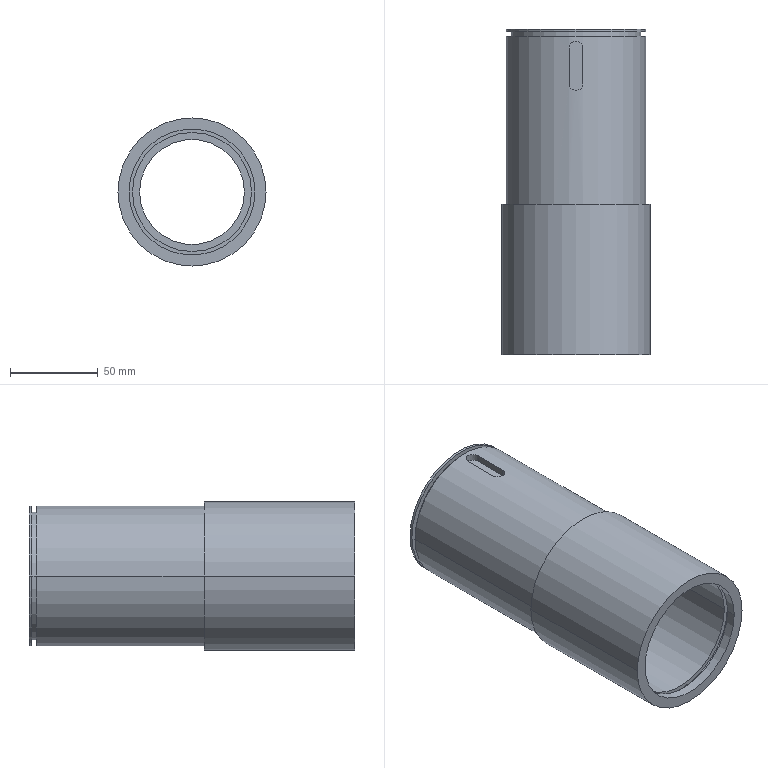Part | SolidWorks | features BaseBody 1 | 1 solid | 32 faces | box 84.6 x 186 x 84.6 mm | volume 291294 mm3 | cylinder 20 | plane 12 | commonest cylinder face diameters 72 x4 80 x4 8 x2 60 x2 68 x2 74 x2
STEP:
#1=CARTESIAN_POINT('',(34.,60.,0.));
#2=VERTEX_POINT('',#1);
#3=CARTESIAN_POINT('',(-34.,60.,0.));
#4=VERTEX_POINT('',#3);
#5=CARTESIAN_POINT('',(0.,60.,0.));
#6=DIRECTION('',(0.,1.,0.));
#7=DIRECTION('',(-1.,0.,0.));
#8=AXIS2_PLACEMENT_3D('',#5,#6,#7);
#9=CIRCLE('',#8,34.);
#10=EDGE_CURVE('',#2,#4,#9,.T.);
#11=ORIENTED_EDGE('',*,*,#10,.F.);
#12=CARTESIAN_POINT('',(34.,172.,0.));
#13=VERTEX_POINT('',#12);
#14=CARTESIAN_POINT('',(34.,0.,0.));
#15=DIRECTION('',(0.,1.,0.));
#16=VECTOR('',#15,1000.);
#17=LINE('',#14,#16);
#18=EDGE_CURVE('',#2,#13,#17,.T.);
#19=ORIENTED_EDGE('',*,*,#18,.T.);
#20=CARTESIAN_POINT('',(-34.,172.,0.));
#21=VERTEX_POINT('',#20);
#22=CARTESIAN_POINT('',(0.,172.,0.));
#23=DIRECTION('',(0.,-1.,0.));
#24=DIRECTION('',(-1.,0.,0.));
#25=AXIS2_PLACEMENT_3D('',#22,#23,#24);
#26=CIRCLE('',#25,34.);
#27=EDGE_CURVE('',#21,#13,#26,.T.);
#28=ORIENTED_EDGE('',*,*,#27,.F.);
#29=CARTESIAN_POINT('',(-34.,0.,0.));
#30=DIRECTION('',(0.,1.,0.));
#31=VECTOR('',#30,1000.);
#32=LINE('',#29,#31);
#33=EDGE_CURVE('',#4,#21,#32,.T.);
#34=ORIENTED_EDGE('',*,*,#33,.F.);
#35=EDGE_LOOP('',(#11,#19,#28,#34));
#36=FACE_OUTER_BOUND('',#35,.T.);
#37=CARTESIAN_POINT('',(0.,0.,0.));
#38=DIRECTION('',(0.,1.,0.));
#39=DIRECTION('',(-1.,0.,0.));
#40=AXIS2_PLACEMENT_3D('',#37,#38,#39);
#41=CYLINDRICAL_SURFACE('',#40,34.);
#42=ADVANCED_FACE('',(#36),#41,.F.);
#43=CARTESIAN_POINT('',(-36.,60.,0.));
#44=VERTEX_POINT('',#43);
#45=CARTESIAN_POINT('',(36.,60.,0.));
#46=VERTEX_POINT('',#45);
#47=CARTESIAN_POINT('',(0.,60.,0.));
#48=DIRECTION('',(0.,-1.,0.));
#49=DIRECTION('',(1.,0.,0.));
#50=AXIS2_PLACEMENT_3D('',#47,#48,#49);
#51=CIRCLE('',#50,36.);
#52=EDGE_CURVE('',#44,#46,#51,.T.);
#53=ORIENTED_EDGE('',*,*,#52,.F.);
#54=CARTESIAN_POINT('',(-36.,8.,0.));
#55=VERTEX_POINT('',#54);
#56=CARTESIAN_POINT('',(-36.,60.,0.));
#57=DIRECTION('',(0.,-1.,0.));
#58=VECTOR('',#57,1000.);
#59=LINE('',#56,#58);
#60=EDGE_CURVE('',#44,#55,#59,.T.);
#61=ORIENTED_EDGE('',*,*,#60,.T.);
#62=CARTESIAN_POINT('',(36.,8.,0.));
#63=VERTEX_POINT('',#62);
#64=CARTESIAN_POINT('',(0.,8.,0.));
#65=DIRECTION('',(0.,1.,0.));
#66=DIRECTION('',(1.,0.,0.));
#67=AXIS2_PLACEMENT_3D('',#64,#65,#66);
#68=CIRCLE('',#67,36.);
#69=EDGE_CURVE('',#63,#55,#68,.T.);
#70=ORIENTED_EDGE('',*,*,#69,.F.);
#71=CARTESIAN_POINT('',(36.,60.,0.));
#72=DIRECTION('',(0.,-1.,0.));
#73=VECTOR('',#72,1000.);
#74=LINE('',#71,#73);
#75=EDGE_CURVE('',#46,#63,#74,.T.);
#76=ORIENTED_EDGE('',*,*,#75,.F.);
#77=EDGE_LOOP('',(#53,#61,#70,#76));
#78=FACE_OUTER_BOUND('',#77,.T.);
#79=CARTESIAN_POINT('',(0.,60.,0.));
#80=DIRECTION('',(0.,-1.,0.));
#81=DIRECTION('',(1.,0.,0.));
#82=AXIS2_PLACEMENT_3D('',#79,#80,#81);
#83=CYLINDRICAL_SURFACE('',#82,36.);
#84=ADVANCED_FACE('',(#78),#83,.F.);
#85=CARTESIAN_POINT('',(-30.,172.,0.));
#86=VERTEX_POINT('',#85);
#87=CARTESIAN_POINT('',(30.,172.,0.));
#88=VERTEX_POINT('',#87);
#89=CARTESIAN_POINT('',(0.,172.,0.));
#90=DIRECTION('',(0.,-1.,0.));
#91=DIRECTION('',(-1.,0.,0.));
#92=AXIS2_PLACEMENT_3D('',#89,#90,#91);
#93=CIRCLE('',#92,30.);
#94=EDGE_CURVE('',#86,#88,#93,.T.);
#95=ORIENTED_EDGE('',*,*,#94,.T.);
#96=CARTESIAN_POINT('',(30.,186.,0.));
#97=VERTEX_POINT('',#96);
#98=CARTESIAN_POINT('',(30.,87.,0.));
#99=DIRECTION('',(0.,1.,0.));
#100=VECTOR('',#99,1000.);
#101=LINE('',#98,#100);
#102=EDGE_CURVE('',#88,#97,#101,.T.);
#103=ORIENTED_EDGE('',*,*,#102,.T.);
#104=CARTESIAN_POINT('',(-30.,186.,0.));
#105=VERTEX_POINT('',#104);
#106=CARTESIAN_POINT('',(0.,186.,0.));
#107=DIRECTION('',(0.,-1.,0.));
#108=DIRECTION('',(-1.,0.,0.));
#109=AXIS2_PLACEMENT_3D('',#106,#107,#108);
#110=CIRCLE('',#109,30.);
#111=EDGE_CURVE('',#105,#97,#110,.T.);
#112=ORIENTED_EDGE('',*,*,#111,.F.);
#113=CARTESIAN_POINT('',(-30.,87.,0.));
#114=DIRECTION('',(0.,1.,0.));
#115=VECTOR('',#114,1000.);
#116=LINE('',#113,#115);
#117=EDGE_CURVE('',#86,#105,#116,.T.);
#118=ORIENTED_EDGE('',*,*,#117,.F.);
#119=EDGE_LOOP('',(#95,#103,#112,#118));
#120=FACE_OUTER_BOUND('',#119,.T.);
#121=CARTESIAN_POINT('',(0.,87.,0.));
#122=DIRECTION('',(0.,1.,0.));
#123=DIRECTION('',(-1.,0.,0.));
#124=AXIS2_PLACEMENT_3D('',#121,#122,#123);
#125=CYLINDRICAL_SURFACE('',#124,30.);
#126=ADVANCED_FACE('',(#120),#125,.F.);
#127=CARTESIAN_POINT('',(38.5,5.4,0.));
#128=VERTEX_POINT('',#127);
#129=CARTESIAN_POINT('',(-38.5,5.4,0.));
#130=VERTEX_POINT('',#129);
#131=CARTESIAN_POINT('',(0.,5.4,0.));
#132=DIRECTION('',(0.,1.,0.));
#133=DIRECTION('',(-1.,0.,0.));
#134=AXIS2_PLACEMENT_3D('',#131,#132,#133);
#135=CIRCLE('',#134,38.5);
#136=EDGE_CURVE('',#128,#130,#135,.T.);
#137=ORIENTED_EDGE('',*,*,#136,.F.);
#138=CARTESIAN_POINT('',(38.5,8.,0.));
#139=VERTEX_POINT('',#138);
#140=CARTESIAN_POINT('',(38.5,5.4,0.));
#141=DIRECTION('',(0.,1.,0.));
#142=VECTOR('',#141,1000.);
#143=LINE('',#140,#142);
#144=EDGE_CURVE('',#128,#139,#143,.T.);
#145=ORIENTED_EDGE('',*,*,#144,.T.);
#146=CARTESIAN_POINT('',(-38.5,8.,0.));
#147=VERTEX_POINT('',#146);
#148=CARTESIAN_POINT('',(0.,8.,0.));
#149=DIRECTION('',(0.,-1.,0.));
#150=DIRECTION('',(-1.,0.,0.));
#151=AXIS2_PLACEMENT_3D('',#148,#149,#150);
#152=CIRCLE('',#151,38.5);
#153=EDGE_CURVE('',#147,#139,#152,.T.);
#154=ORIENTED_EDGE('',*,*,#153,.F.);
#155=CARTESIAN_POINT('',(-38.5,5.4,0.));
#156=DIRECTION('',(0.,1.,0.));
#157=VECTOR('',#156,1000.);
#158=LINE('',#155,#157);
#159=EDGE_CURVE('',#130,#147,#158,.T.);
#160=ORIENTED_EDGE('',*,*,#159,.F.);
#161=EDGE_LOOP('',(#137,#145,#154,#160));
#162=FACE_OUTER_BOUND('',#161,.T.);
#163=CARTESIAN_POINT('',(0.,5.4,0.));
#164=DIRECTION('',(0.,1.,0.));
#165=DIRECTION('',(-1.,0.,0.));
#166=AXIS2_PLACEMENT_3D('',#163,#164,#165);
#167=CYLINDRICAL_SURFACE('',#166,38.5);
#168=ADVANCED_FACE('',(#162),#167,.F.);
#169=CARTESIAN_POINT('',(-40.,186.,0.));
#170=VERTEX_POINT('',#169);
#171=CARTESIAN_POINT('',(40.,186.,0.));
#172=VERTEX_POINT('',#171);
#173=CARTESIAN_POINT('',(0.,186.,0.));
#174=DIRECTION('',(0.,1.,0.));
#175=DIRECTION('',(1.,0.,0.));
#176=AXIS2_PLACEMENT_3D('',#173,#174,#175);
#177=CIRCLE('',#176,40.);
#178=EDGE_CURVE('',#170,#172,#177,.T.);
#179=ORIENTED_EDGE('',*,*,#178,.F.);
#180=CARTESIAN_POINT('',(-40.,184.5,0.));
#181=VERTEX_POINT('',#180);
#182=CARTESIAN_POINT('',(-40.,186.,0.));
#183=DIRECTION('',(0.,-1.,0.));
#184=VECTOR('',#183,1000.);
#185=LINE('',#182,#184);
#186=EDGE_CURVE('',#170,#181,#185,.T.);
#187=ORIENTED_EDGE('',*,*,#186,.T.);
#188=CARTESIAN_POINT('',(40.,184.5,0.));
#189=VERTEX_POINT('',#188);
#190=CARTESIAN_POINT('',(0.,184.5,0.));
#191=DIRECTION('',(0.,1.,0.));
#192=DIRECTION('',(1.,0.,0.));
#193=AXIS2_PLACEMENT_3D('',#190,#191,#192);
#194=CIRCLE('',#193,40.);
#195=EDGE_CURVE('',#181,#189,#194,.T.);
#196=ORIENTED_EDGE('',*,*,#195,.T.);
#197=CARTESIAN_POINT('',(40.,186.,0.));
#198=DIRECTION('',(0.,-1.,0.));
#199=VECTOR('',#198,1000.);
#200=LINE('',#197,#199);
#201=EDGE_CURVE('',#172,#189,#200,.T.);
#202=ORIENTED_EDGE('',*,*,#201,.F.);
#203=EDGE_LOOP('',(#179,#187,#196,#202));
#204=FACE_OUTER_BOUND('',#203,.T.);
#205=CARTESIAN_POINT('',(0.,186.,0.));
#206=DIRECTION('',(0.,-1.,0.));
#207=DIRECTION('',(1.,0.,0.));
#208=AXIS2_PLACEMENT_3D('',#205,#206,#207);
#209=CYLINDRICAL_SURFACE('',#208,40.);
#210=ADVANCED_FACE('',(#204),#209,.T.);
#211=CARTESIAN_POINT('',(36.,5.4,0.));
#212=VERTEX_POINT('',#211);
#213=CARTESIAN_POINT('',(-36.,5.4,0.));
#214=VERTEX_POINT('',#213);
#215=CARTESIAN_POINT('',(0.,5.4,0.));
#216=DIRECTION('',(0.,1.,0.));
#217=DIRECTION('',(1.,0.,0.));
#218=AXIS2_PLACEMENT_3D('',#215,#216,#217);
#219=CIRCLE('',#218,36.);
#220=EDGE_CURVE('',#212,#214,#219,.T.);
#221=ORIENTED_EDGE('',*,*,#220,.T.);
#222=CARTESIAN_POINT('',(-36.,0.,0.));
#223=VERTEX_POINT('',#222);
#224=CARTESIAN_POINT('',(-36.,60.,0.));
#225=DIRECTION('',(0.,-1.,0.));
#226=VECTOR('',#225,1000.);
#227=LINE('',#224,#226);
#228=EDGE_CURVE('',#214,#223,#227,.T.);
#229=ORIENTED_EDGE('',*,*,#228,.T.);
#230=CARTESIAN_POINT('',(36.,0.,0.));
#231=VERTEX_POINT('',#230);
#232=CARTESIAN_POINT('',(0.,0.,0.));
#233=DIRECTION('',(0.,1.,0.));
#234=DIRECTION('',(1.,0.,0.));
#235=AXIS2_PLACEMENT_3D('',#232,#233,#234);
#236=CIRCLE('',#235,36.);
#237=EDGE_CURVE('',#231,#223,#236,.T.);
#238=ORIENTED_EDGE('',*,*,#237,.F.);
#239=CARTESIAN_POINT('',(36.,60.,0.));
#240=DIRECTION('',(0.,-1.,0.));
#241=VECTOR('',#240,1000.);
#242=LINE('',#239,#241);
#243=EDGE_CURVE('',#212,#231,#242,.T.);
#244=ORIENTED_EDGE('',*,*,#243,.F.);
#245=EDGE_LOOP('',(#221,#229,#238,#244));
#246=FACE_OUTER_BOUND('',#245,.T.);
#247=CARTESIAN_POINT('',(0.,60.,0.));
#248=DIRECTION('',(0.,-1.,0.));
#249=DIRECTION('',(1.,0.,0.));
#250=AXIS2_PLACEMENT_3D('',#247,#248,#249);
#251=CYLINDRICAL_SURFACE('',#250,36.);
#252=ADVANCED_FACE('',(#246),#251,.F.);
#253=CARTESIAN_POINT('',(-37.,182.,0.));
#254=VERTEX_POINT('',#253);
#255=CARTESIAN_POINT('',(37.,182.,0.));
#256=VERTEX_POINT('',#255);
#257=CARTESIAN_POINT('',(0.,182.,0.));
#258=DIRECTION('',(0.,1.,0.));
#259=DIRECTION('',(-1.,0.,0.));
#260=AXIS2_PLACEMENT_3D('',#257,#258,#259);
#261=CIRCLE('',#260,37.);
#262=EDGE_CURVE('',#254,#256,#261,.T.);
#263=ORIENTED_EDGE('',*,*,#262,.T.);
#264=CARTESIAN_POINT('',(37.,184.5,0.));
#265=VERTEX_POINT('',#264);
#266=CARTESIAN_POINT('',(37.,182.,0.));
#267=DIRECTION('',(0.,1.,0.));
#268=VECTOR('',#267,1000.);
#269=LINE('',#266,#268);
#270=EDGE_CURVE('',#256,#265,#269,.T.);
#271=ORIENTED_EDGE('',*,*,#270,.T.);
#272=CARTESIAN_POINT('',(-37.,184.5,0.));
#273=VERTEX_POINT('',#272);
#274=CARTESIAN_POINT('',(0.,184.5,0.));
#275=DIRECTION('',(0.,-1.,0.));
#276=DIRECTION('',(-1.,0.,0.));
#277=AXIS2_PLACEMENT_3D('',#274,#275,#276);
#278=CIRCLE('',#277,37.);
#279=EDGE_CURVE('',#265,#273,#278,.T.);
#280=ORIENTED_EDGE('',*,*,#279,.T.);
#281=CARTESIAN_POINT('',(-37.,182.,0.));
#282=DIRECTION('',(0.,1.,0.));
#283=VECTOR('',#282,1000.);
#284=LINE('',#281,#283);
#285=EDGE_CURVE('',#254,#273,#284,.T.);
#286=ORIENTED_EDGE('',*,*,#285,.F.);
#287=EDGE_LOOP('',(#263,#271,#280,#286));
#288=FACE_OUTER_BOUND('',#287,.T.);
#289=CARTESIAN_POINT('',(0.,182.,0.));
#290=DIRECTION('',(0.,1.,0.));
#291=DIRECTION('',(-1.,0.,0.));
#292=AXIS2_PLACEMENT_3D('',#289,#290,#291);
#293=CYLINDRICAL_SURFACE('',#292,37.);
#294=ADVANCED_FACE('',(#288),#293,.T.);
#295=CARTESIAN_POINT('',(42.3,86.,0.));
#296=VERTEX_POINT('',#295);
#297=CARTESIAN_POINT('',(-42.3,86.,0.));
#298=VERTEX_POINT('',#297);
#299=CARTESIAN_POINT('',(0.,86.,0.));
#300=DIRECTION('',(0.,-1.,0.));
#301=DIRECTION('',(1.,0.,0.));
#302=AXIS2_PLACEMENT_3D('',#299,#300,#301);
#303=CIRCLE('',#302,42.3);
#304=EDGE_CURVE('',#296,#298,#303,.T.);
#305=ORIENTED_EDGE('',*,*,#304,.T.);
#306=CARTESIAN_POINT('',(-42.3,0.,0.));
#307=VERTEX_POINT('',#306);
#308=CARTESIAN_POINT('',(-42.3,86.,0.));
#309=DIRECTION('',(0.,-1.,0.));
#310=VECTOR('',#309,1000.);
#311=LINE('',#308,#310);
#312=EDGE_CURVE('',#298,#307,#311,.T.);
#313=ORIENTED_EDGE('',*,*,#312,.T.);
#314=CARTESIAN_POINT('',(42.3,0.,0.));
#315=VERTEX_POINT('',#314);
#316=CARTESIAN_POINT('',(0.,0.,0.));
#317=DIRECTION('',(0.,1.,0.));
#318=DIRECTION('',(1.,0.,0.));
#319=AXIS2_PLACEMENT_3D('',#316,#317,#318);
#320=CIRCLE('',#319,42.3);
#321=EDGE_CURVE('',#307,#315,#320,.T.);
#322=ORIENTED_EDGE('',*,*,#321,.T.);
#323=CARTESIAN_POINT('',(42.3,86.,0.));
#324=DIRECTION('',(0.,-1.,0.));
#325=VECTOR('',#324,1000.);
#326=LINE('',#323,#325);
#327=EDGE_CURVE('',#296,#315,#326,.T.);
#328=ORIENTED_EDGE('',*,*,#327,.F.);
#329=EDGE_LOOP('',(#305,#313,#322,#328));
#330=FACE_OUTER_BOUND('',#329,.T.);
#331=CARTESIAN_POINT('',(0.,86.,0.));
#332=DIRECTION('',(0.,-1.,0.));
#333=DIRECTION('',(1.,0.,0.));
#334=AXIS2_PLACEMENT_3D('',#331,#332,#333);
#335=CYLINDRICAL_SURFACE('',#334,42.3);
#336=ADVANCED_FACE('',(#330),#335,.T.);
#337=CARTESIAN_POINT('',(-4.,155.,39.799));
#338=VERTEX_POINT('',#337);
#339=CARTESIAN_POINT('',(-4.,175.,39.799));
#340=VERTEX_POINT('',#339);
#341=CARTESIAN_POINT('',(-4.,186.,39.799));
#342=DIRECTION('',(0.,1.,0.));
#343=VECTOR('',#342,1000.);
#344=LINE('',#341,#343);
#345=EDGE_CURVE('',#338,#340,#344,.T.);
#346=ORIENTED_EDGE('',*,*,#345,.T.);
#347=CARTESIAN_POINT('',(4.,175.,39.799));
#348=VERTEX_POINT('',#347);
#349=CARTESIAN_POINT('',(-4.,175.,39.799));
#350=CARTESIAN_POINT('',(-4.,175.264,39.799));
#351=CARTESIAN_POINT('',(-3.974,175.524,39.802));
#352=CARTESIAN_POINT('',(-3.872,176.035,39.812));
#353=CARTESIAN_POINT('',(-3.796,176.289,39.82));
#354=CARTESIAN_POINT('',(-3.595,176.773,39.838));
#355=CARTESIAN_POINT('',(-3.472,177.003,39.849));
#356=CARTESIAN_POINT('',(-3.182,177.437,39.873));
#357=CARTESIAN_POINT('',(-3.014,177.643,39.887));
#358=CARTESIAN_POINT('',(-2.645,178.012,39.913));
#359=CARTESIAN_POINT('',(-2.444,178.177,39.926));
#360=CARTESIAN_POINT('',(-2.007,178.47,39.95));
#361=CARTESIAN_POINT('',(-1.775,178.594,39.961));
#362=CARTESIAN_POINT('',(-1.294,178.794,39.98));
#363=CARTESIAN_POINT('',(-1.042,178.871,39.987));
#364=CARTESIAN_POINT('',(-0.5256,178.974,39.997));
#365=CARTESIAN_POINT('',(-0.2643,179.,40.));
#366=CARTESIAN_POINT('',(0.2643,179.,40.));
#367=CARTESIAN_POINT('',(0.5241,178.974,39.997));
#368=CARTESIAN_POINT('',(1.035,178.872,39.987));
#369=CARTESIAN_POINT('',(1.289,178.796,39.98));
#370=CARTESIAN_POINT('',(1.773,178.595,39.961));
#371=CARTESIAN_POINT('',(2.003,178.472,39.95));
#372=CARTESIAN_POINT('',(2.437,178.182,39.926));
#373=CARTESIAN_POINT('',(2.643,178.014,39.913));
#374=CARTESIAN_POINT('',(3.012,177.645,39.887));
#375=CARTESIAN_POINT('',(3.177,177.444,39.874));
#376=CARTESIAN_POINT('',(3.47,177.007,39.849));
#377=CARTESIAN_POINT('',(3.594,176.775,39.838));
#378=CARTESIAN_POINT('',(3.794,176.294,39.82));
#379=CARTESIAN_POINT('',(3.871,176.042,39.812));
#380=CARTESIAN_POINT('',(3.974,175.526,39.802));
#381=CARTESIAN_POINT('',(4.,175.264,39.799));
#382=CARTESIAN_POINT('',(4.,175.,39.799));
#383=B_SPLINE_CURVE_WITH_KNOTS('',3,(#349,#350,#351,#352,#353,#354,#355,#356,#357,#358,#359,#360,#361,#362,#363,#364,#365,#366,#367,#368,#369,#370,#371,#372,#373,#374,#375,#376,#377,#378,#379,#380,#381,#382),.UNSPECIFIED.,.F.,.F.,(4,2,2,2,2,2,2,2,2,2,2,2,2,2,2,2,4),(-0.006252,-0.005471,-0.004689,-0.003908,-0.003126,-0.002345,-0.001563,-0.0007815,0.000000023,0.0007816,0.001563,0.002345,0.003126,0.003908,0.004689,0.005471,0.006253),.UNSPECIFIED.);
#384=EDGE_CURVE('',#340,#348,#383,.T.);
#385=ORIENTED_EDGE('',*,*,#384,.T.);
#386=CARTESIAN_POINT('',(4.,155.,39.799));
#387=VERTEX_POINT('',#386);
#388=CARTESIAN_POINT('',(4.,186.,39.799));
#389=DIRECTION('',(0.,-1.,0.));
#390=VECTOR('',#389,1000.);
#391=LINE('',#388,#390);
#392=EDGE_CURVE('',#348,#387,#391,.T.);
#393=ORIENTED_EDGE('',*,*,#392,.T.);
#394=CARTESIAN_POINT('',(4.,155.,39.799));
#395=CARTESIAN_POINT('',(4.,154.736,39.799));
#396=CARTESIAN_POINT('',(3.974,154.476,39.802));
#397=CARTESIAN_POINT('',(3.872,153.965,39.812));
#398=CARTESIAN_POINT('',(3.796,153.711,39.82));
#399=CARTESIAN_POINT('',(3.595,153.227,39.838));
#400=CARTESIAN_POINT('',(3.472,152.997,39.849));
#401=CARTESIAN_POINT('',(3.182,152.563,39.873));
#402=CARTESIAN_POINT('',(3.014,152.357,39.887));
#403=CARTESIAN_POINT('',(2.645,151.988,39.913));
#404=CARTESIAN_POINT('',(2.444,151.823,39.926));
#405=CARTESIAN_POINT('',(2.007,151.53,39.95));
#406=CARTESIAN_POINT('',(1.775,151.406,39.961));
#407=CARTESIAN_POINT('',(1.294,151.206,39.98));
#408=CARTESIAN_POINT('',(1.042,151.129,39.987));
#409=CARTESIAN_POINT('',(0.5256,151.026,39.997));
#410=CARTESIAN_POINT('',(0.2643,151.,40.));
#411=CARTESIAN_POINT('',(-0.2643,151.,40.));
#412=CARTESIAN_POINT('',(-0.5241,151.026,39.997));
#413=CARTESIAN_POINT('',(-1.035,151.128,39.987));
#414=CARTESIAN_POINT('',(-1.289,151.204,39.98));
#415=CARTESIAN_POINT('',(-1.773,151.405,39.961));
#416=CARTESIAN_POINT('',(-2.003,151.528,39.95));
#417=CARTESIAN_POINT('',(-2.437,151.818,39.926));
#418=CARTESIAN_POINT('',(-2.643,151.986,39.913));
#419=CARTESIAN_POINT('',(-3.012,152.355,39.887));
#420=CARTESIAN_POINT('',(-3.177,152.556,39.874));
#421=CARTESIAN_POINT('',(-3.47,152.993,39.849));
#422=CARTESIAN_POINT('',(-3.594,153.225,39.838));
#423=CARTESIAN_POINT('',(-3.794,153.706,39.82));
#424=CARTESIAN_POINT('',(-3.871,153.958,39.812));
#425=CARTESIAN_POINT('',(-3.974,154.474,39.802));
#426=CARTESIAN_POINT('',(-4.,154.736,39.799));
#427=CARTESIAN_POINT('',(-4.,155.,39.799));
#428=B_SPLINE_CURVE_WITH_KNOTS('',3,(#394,#395,#396,#397,#398,#399,#400,#401,#402,#403,#404,#405,#406,#407,#408,#409,#410,#411,#412,#413,#414,#415,#416,#417,#418,#419,#420,#421,#422,#423,#424,#425,#426,#427),.UNSPECIFIED.,.F.,.F.,(4,2,2,2,2,2,2,2,2,2,2,2,2,2,2,2,4),(0.,0.0007816,0.001563,0.002345,0.003126,0.003908,0.004689,0.005471,0.006253,0.007034,0.007816,0.008597,0.009379,0.01016,0.01094,0.01172,0.01251),.UNSPECIFIED.);
#429=EDGE_CURVE('',#387,#338,#428,.T.);
#430=ORIENTED_EDGE('',*,*,#429,.T.);
#431=EDGE_LOOP('',(#346,#385,#393,#430));
#432=FACE_BOUND('',#431,.T.);
#433=CARTESIAN_POINT('',(-40.,182.,0.));
#434=VERTEX_POINT('',#433);
#435=CARTESIAN_POINT('',(40.,182.,0.));
#436=VERTEX_POINT('',#435);
#437=CARTESIAN_POINT('',(0.,182.,0.));
#438=DIRECTION('',(0.,1.,0.));
#439=DIRECTION('',(1.,0.,0.));
#440=AXIS2_PLACEMENT_3D('',#437,#438,#439);
#441=CIRCLE('',#440,40.);
#442=EDGE_CURVE('',#434,#436,#441,.T.);
#443=ORIENTED_EDGE('',*,*,#442,.F.);
#444=CARTESIAN_POINT('',(-40.,86.,0.));
#445=VERTEX_POINT('',#444);
#446=CARTESIAN_POINT('',(-40.,186.,0.));
#447=DIRECTION('',(0.,-1.,0.));
#448=VECTOR('',#447,1000.);
#449=LINE('',#446,#448);
#450=EDGE_CURVE('',#434,#445,#449,.T.);
#451=ORIENTED_EDGE('',*,*,#450,.T.);
#452=CARTESIAN_POINT('',(40.,86.,0.));
#453=VERTEX_POINT('',#452);
#454=CARTESIAN_POINT('',(0.,86.,0.));
#455=DIRECTION('',(0.,1.,0.));
#456=DIRECTION('',(1.,0.,0.));
#457=AXIS2_PLACEMENT_3D('',#454,#455,#456);
#458=CIRCLE('',#457,40.);
#459=EDGE_CURVE('',#445,#453,#458,.T.);
#460=ORIENTED_EDGE('',*,*,#459,.T.);
#461=CARTESIAN_POINT('',(40.,186.,0.));
#462=DIRECTION('',(0.,-1.,0.));
#463=VECTOR('',#462,1000.);
#464=LINE('',#461,#463);
#465=EDGE_CURVE('',#436,#453,#464,.T.);
#466=ORIENTED_EDGE('',*,*,#465,.F.);
#467=EDGE_LOOP('',(#443,#451,#460,#466));
#468=FACE_OUTER_BOUND('',#467,.T.);
#469=CARTESIAN_POINT('',(0.,186.,0.));
#470=DIRECTION('',(0.,-1.,0.));
#471=DIRECTION('',(1.,0.,0.));
#472=AXIS2_PLACEMENT_3D('',#469,#470,#471);
#473=CYLINDRICAL_SURFACE('',#472,40.);
#474=ADVANCED_FACE('',(#432,#468),#473,.T.);
#475=ORIENTED_EDGE('',*,*,#18,.F.);
#476=CARTESIAN_POINT('',(0.,60.,0.));
#477=DIRECTION('',(0.,1.,0.));
#478=DIRECTION('',(-1.,0.,0.));
#479=AXIS2_PLACEMENT_3D('',#476,#477,#478);
#480=CIRCLE('',#479,34.);
#481=EDGE_CURVE('',#4,#2,#480,.T.);
#482=ORIENTED_EDGE('',*,*,#481,.F.);
#483=ORIENTED_EDGE('',*,*,#33,.T.);
#484=CARTESIAN_POINT('',(0.,172.,0.));
#485=DIRECTION('',(0.,-1.,0.));
#486=DIRECTION('',(-1.,0.,0.));
#487=AXIS2_PLACEMENT_3D('',#484,#485,#486);
#488=CIRCLE('',#487,34.);
#489=EDGE_CURVE('',#13,#21,#488,.T.);
#490=ORIENTED_EDGE('',*,*,#489,.F.);
#491=EDGE_LOOP('',(#475,#482,#483,#490));
#492=FACE_OUTER_BOUND('',#491,.T.);
#493=CARTESIAN_POINT('',(0.,0.,0.));
#494=DIRECTION('',(0.,1.,0.));
#495=DIRECTION('',(-1.,0.,0.));
#496=AXIS2_PLACEMENT_3D('',#493,#494,#495);
#497=CYLINDRICAL_SURFACE('',#496,34.);
#498=ADVANCED_FACE('',(#492),#497,.F.);
#499=ORIENTED_EDGE('',*,*,#481,.T.);
#500=ORIENTED_EDGE('',*,*,#10,.T.);
#501=EDGE_LOOP('',(#499,#500));
#502=FACE_BOUND('',#501,.T.);
#503=CARTESIAN_POINT('',(0.,60.,0.));
#504=DIRECTION('',(0.,-1.,0.));
#505=DIRECTION('',(1.,0.,0.));
#506=AXIS2_PLACEMENT_3D('',#503,#504,#505);
#507=CIRCLE('',#506,36.);
#508=EDGE_CURVE('',#46,#44,#507,.T.);
#509=ORIENTED_EDGE('',*,*,#508,.T.);
#510=ORIENTED_EDGE('',*,*,#52,.T.);
#511=EDGE_LOOP('',(#509,#510));
#512=FACE_OUTER_BOUND('',#511,.T.);
#513=CARTESIAN_POINT('',(0.,60.,0.));
#514=DIRECTION('',(0.,-1.,0.));
#515=DIRECTION('',(1.,0.,0.));
#516=AXIS2_PLACEMENT_3D('',#513,#514,#515);
#517=PLANE('',#516);
#518=ADVANCED_FACE('',(#502,#512),#517,.T.);
#519=ORIENTED_EDGE('',*,*,#94,.F.);
#520=CARTESIAN_POINT('',(0.,172.,0.));
#521=DIRECTION('',(0.,-1.,0.));
#522=DIRECTION('',(-1.,0.,0.));
#523=AXIS2_PLACEMENT_3D('',#520,#521,#522);
#524=CIRCLE('',#523,30.);
#525=EDGE_CURVE('',#88,#86,#524,.T.);
#526=ORIENTED_EDGE('',*,*,#525,.F.);
#527=EDGE_LOOP('',(#519,#526));
#528=FACE_BOUND('',#527,.T.);
#529=ORIENTED_EDGE('',*,*,#27,.T.);
#530=ORIENTED_EDGE('',*,*,#489,.T.);
#531=EDGE_LOOP('',(#529,#530));
#532=FACE_OUTER_BOUND('',#531,.T.);
#533=CARTESIAN_POINT('',(0.,172.,0.));
#534=DIRECTION('',(0.,1.,0.));
#535=DIRECTION('',(-1.,0.,0.));
#536=AXIS2_PLACEMENT_3D('',#533,#534,#535);
#537=PLANE('',#536);
#538=ADVANCED_FACE('',(#528,#532),#537,.F.);
#539=ORIENTED_EDGE('',*,*,#60,.F.);
#540=ORIENTED_EDGE('',*,*,#508,.F.);
#541=ORIENTED_EDGE('',*,*,#75,.T.);
#542=CARTESIAN_POINT('',(0.,8.,0.));
#543=DIRECTION('',(0.,1.,0.));
#544=DIRECTION('',(1.,0.,0.));
#545=AXIS2_PLACEMENT_3D('',#542,#543,#544);
#546=CIRCLE('',#545,36.);
#547=EDGE_CURVE('',#55,#63,#546,.T.);
#548=ORIENTED_EDGE('',*,*,#547,.F.);
#549=EDGE_LOOP('',(#539,#540,#541,#548));
#550=FACE_OUTER_BOUND('',#549,.T.);
#551=CARTESIAN_POINT('',(0.,60.,0.));
#552=DIRECTION('',(0.,-1.,0.));
#553=DIRECTION('',(1.,0.,0.));
#554=AXIS2_PLACEMENT_3D('',#551,#552,#553);
#555=CYLINDRICAL_SURFACE('',#554,36.);
#556=ADVANCED_FACE('',(#550),#555,.F.);
#557=ORIENTED_EDGE('',*,*,#102,.F.);
#558=ORIENTED_EDGE('',*,*,#525,.T.);
#559=ORIENTED_EDGE('',*,*,#117,.T.);
#560=CARTESIAN_POINT('',(0.,186.,0.));
#561=DIRECTION('',(0.,-1.,0.));
#562=DIRECTION('',(-1.,0.,0.));
#563=AXIS2_PLACEMENT_3D('',#560,#561,#562);
#564=CIRCLE('',#563,30.);
#565=EDGE_CURVE('',#97,#105,#564,.T.);
#566=ORIENTED_EDGE('',*,*,#565,.F.);
#567=EDGE_LOOP('',(#557,#558,#559,#566));
#568=FACE_OUTER_BOUND('',#567,.T.);
#569=CARTESIAN_POINT('',(0.,87.,0.));
#570=DIRECTION('',(0.,1.,0.));
#571=DIRECTION('',(-1.,0.,0.));
#572=AXIS2_PLACEMENT_3D('',#569,#570,#571);
#573=CYLINDRICAL_SURFACE('',#572,30.);
#574=ADVANCED_FACE('',(#568),#573,.F.);
#575=ORIENTED_EDGE('',*,*,#69,.T.);
#576=ORIENTED_EDGE('',*,*,#547,.T.);
#577=EDGE_LOOP('',(#575,#576));
#578=FACE_BOUND('',#577,.T.);
#579=ORIENTED_EDGE('',*,*,#153,.T.);
#580=CARTESIAN_POINT('',(0.,8.,0.));
#581=DIRECTION('',(0.,-1.,0.));
#582=DIRECTION('',(-1.,0.,0.));
#583=AXIS2_PLACEMENT_3D('',#580,#581,#582);
#584=CIRCLE('',#583,38.5);
#585=EDGE_CURVE('',#139,#147,#584,.T.);
#586=ORIENTED_EDGE('',*,*,#585,.T.);
#587=EDGE_LOOP('',(#579,#586));
#588=FACE_OUTER_BOUND('',#587,.T.);
#589=CARTESIAN_POINT('',(0.,8.,0.));
#590=DIRECTION('',(0.,-1.,0.));
#591=DIRECTION('',(1.,0.,0.));
#592=AXIS2_PLACEMENT_3D('',#589,#590,#591);
#593=PLANE('',#592);
#594=ADVANCED_FACE('',(#578,#588),#593,.T.);
#595=CARTESIAN_POINT('',(0.,186.,0.));
#596=DIRECTION('',(0.,1.,0.));
#597=DIRECTION('',(1.,0.,0.));
#598=AXIS2_PLACEMENT_3D('',#595,#596,#597);
#599=CIRCLE('',#598,40.);
#600=EDGE_CURVE('',#172,#170,#599,.T.);
#601=ORIENTED_EDGE('',*,*,#600,.T.);
#602=ORIENTED_EDGE('',*,*,#178,.T.);
#603=EDGE_LOOP('',(#601,#602));
#604=FACE_OUTER_BOUND('',#603,.T.);
#605=ORIENTED_EDGE('',*,*,#111,.T.);
#606=ORIENTED_EDGE('',*,*,#565,.T.);
#607=EDGE_LOOP('',(#605,#606));
#608=FACE_BOUND('',#607,.T.);
#609=CARTESIAN_POINT('',(0.,186.,0.));
#610=DIRECTION('',(0.,1.,0.));
#611=DIRECTION('',(-1.,0.,0.));
#612=AXIS2_PLACEMENT_3D('',#609,#610,#611);
#613=PLANE('',#612);
#614=ADVANCED_FACE('',(#604,#608),#613,.T.);
#615=ORIENTED_EDGE('',*,*,#144,.F.);
#616=CARTESIAN_POINT('',(0.,5.4,0.));
#617=DIRECTION('',(0.,1.,0.));
#618=DIRECTION('',(-1.,0.,0.));
#619=AXIS2_PLACEMENT_3D('',#616,#617,#618);
#620=CIRCLE('',#619,38.5);
#621=EDGE_CURVE('',#130,#128,#620,.T.);
#622=ORIENTED_EDGE('',*,*,#621,.F.);
#623=ORIENTED_EDGE('',*,*,#159,.T.);
#624=ORIENTED_EDGE('',*,*,#585,.F.);
#625=EDGE_LOOP('',(#615,#622,#623,#624));
#626=FACE_OUTER_BOUND('',#625,.T.);
#627=CARTESIAN_POINT('',(0.,5.4,0.));
#628=DIRECTION('',(0.,1.,0.));
#629=DIRECTION('',(-1.,0.,0.));
#630=AXIS2_PLACEMENT_3D('',#627,#628,#629);
#631=CYLINDRICAL_SURFACE('',#630,38.5);
#632=ADVANCED_FACE('',(#626),#631,.F.);
#633=ORIENTED_EDGE('',*,*,#186,.F.);
#634=ORIENTED_EDGE('',*,*,#600,.F.);
#635=ORIENTED_EDGE('',*,*,#201,.T.);
#636=CARTESIAN_POINT('',(0.,184.5,0.));
#637=DIRECTION('',(0.,1.,0.));
#638=DIRECTION('',(1.,0.,0.));
#639=AXIS2_PLACEMENT_3D('',#636,#637,#638);
#640=CIRCLE('',#639,40.);
#641=EDGE_CURVE('',#189,#181,#640,.T.);
#642=ORIENTED_EDGE('',*,*,#641,.T.);
#643=EDGE_LOOP('',(#633,#634,#635,#642));
#644=FACE_OUTER_BOUND('',#643,.T.);
#645=CARTESIAN_POINT('',(0.,186.,0.));
#646=DIRECTION('',(0.,-1.,0.));
#647=DIRECTION('',(1.,0.,0.));
#648=AXIS2_PLACEMENT_3D('',#645,#646,#647);
#649=CYLINDRICAL_SURFACE('',#648,40.);
#650=ADVANCED_FACE('',(#644),#649,.T.);
#651=ORIENTED_EDGE('',*,*,#220,.F.);
#652=CARTESIAN_POINT('',(0.,5.4,0.));
#653=DIRECTION('',(0.,1.,0.));
#654=DIRECTION('',(1.,0.,0.));
#655=AXIS2_PLACEMENT_3D('',#652,#653,#654);
#656=CIRCLE('',#655,36.);
#657=EDGE_CURVE('',#214,#212,#656,.T.);
#658=ORIENTED_EDGE('',*,*,#657,.F.);
#659=EDGE_LOOP('',(#651,#658));
#660=FACE_BOUND('',#659,.T.);
#661=ORIENTED_EDGE('',*,*,#621,.T.);
#662=ORIENTED_EDGE('',*,*,#136,.T.);
#663=EDGE_LOOP('',(#661,#662));
#664=FACE_OUTER_BOUND('',#663,.T.);
#665=CARTESIAN_POINT('',(0.,5.4,0.));
#666=DIRECTION('',(0.,-1.,0.));
#667=DIRECTION('',(1.,0.,0.));
#668=AXIS2_PLACEMENT_3D('',#665,#666,#667);
#669=PLANE('',#668);
#670=ADVANCED_FACE('',(#660,#664),#669,.F.);
#671=ORIENTED_EDGE('',*,*,#641,.F.);
#672=ORIENTED_EDGE('',*,*,#195,.F.);
#673=EDGE_LOOP('',(#671,#672));
#674=FACE_OUTER_BOUND('',#673,.T.);
#675=CARTESIAN_POINT('',(0.,184.5,0.));
#676=DIRECTION('',(0.,-1.,0.));
#677=DIRECTION('',(-1.,0.,0.));
#678=AXIS2_PLACEMENT_3D('',#675,#676,#677);
#679=CIRCLE('',#678,37.);
#680=EDGE_CURVE('',#273,#265,#679,.T.);
#681=ORIENTED_EDGE('',*,*,#680,.F.);
#682=ORIENTED_EDGE('',*,*,#279,.F.);
#683=EDGE_LOOP('',(#681,#682));
#684=FACE_BOUND('',#683,.T.);
#685=CARTESIAN_POINT('',(0.,184.5,0.));
#686=DIRECTION('',(0.,1.,0.));
#687=DIRECTION('',(-1.,0.,0.));
#688=AXIS2_PLACEMENT_3D('',#685,#686,#687);
#689=PLANE('',#688);
#690=ADVANCED_FACE('',(#674,#684),#689,.F.);
#691=ORIENTED_EDGE('',*,*,#228,.F.);
#692=ORIENTED_EDGE('',*,*,#657,.T.);
#693=ORIENTED_EDGE('',*,*,#243,.T.);
#694=CARTESIAN_POINT('',(0.,0.,0.));
#695=DIRECTION('',(0.,1.,0.));
#696=DIRECTION('',(1.,0.,0.));
#697=AXIS2_PLACEMENT_3D('',#694,#695,#696);
#698=CIRCLE('',#697,36.);
#699=EDGE_CURVE('',#223,#231,#698,.T.);
#700=ORIENTED_EDGE('',*,*,#699,.F.);
#701=EDGE_LOOP('',(#691,#692,#693,#700));
#702=FACE_OUTER_BOUND('',#701,.T.);
#703=CARTESIAN_POINT('',(0.,60.,0.));
#704=DIRECTION('',(0.,-1.,0.));
#705=DIRECTION('',(1.,0.,0.));
#706=AXIS2_PLACEMENT_3D('',#703,#704,#705);
#707=CYLINDRICAL_SURFACE('',#706,36.);
#708=ADVANCED_FACE('',(#702),#707,.F.);
#709=ORIENTED_EDGE('',*,*,#270,.F.);
#710=CARTESIAN_POINT('',(0.,182.,0.));
#711=DIRECTION('',(0.,1.,0.));
#712=DIRECTION('',(-1.,0.,0.));
#713=AXIS2_PLACEMENT_3D('',#710,#711,#712);
#714=CIRCLE('',#713,37.);
#715=EDGE_CURVE('',#256,#254,#714,.T.);
#716=ORIENTED_EDGE('',*,*,#715,.T.);
#717=ORIENTED_EDGE('',*,*,#285,.T.);
#718=ORIENTED_EDGE('',*,*,#680,.T.);
#719=EDGE_LOOP('',(#709,#716,#717,#718));
#720=FACE_OUTER_BOUND('',#719,.T.);
#721=CARTESIAN_POINT('',(0.,182.,0.));
#722=DIRECTION('',(0.,1.,0.));
#723=DIRECTION('',(-1.,0.,0.));
#724=AXIS2_PLACEMENT_3D('',#721,#722,#723);
#725=CYLINDRICAL_SURFACE('',#724,37.);
#726=ADVANCED_FACE('',(#720),#725,.T.);
#727=CARTESIAN_POINT('',(0.,0.,0.));
#728=DIRECTION('',(0.,1.,0.));
#729=DIRECTION('',(1.,0.,0.));
#730=AXIS2_PLACEMENT_3D('',#727,#728,#729);
#731=CIRCLE('',#730,42.3);
#732=EDGE_CURVE('',#315,#307,#731,.T.);
#733=ORIENTED_EDGE('',*,*,#732,.F.);
#734=ORIENTED_EDGE('',*,*,#321,.F.);
#735=EDGE_LOOP('',(#733,#734));
#736=FACE_OUTER_BOUND('',#735,.T.);
#737=ORIENTED_EDGE('',*,*,#237,.T.);
#738=ORIENTED_EDGE('',*,*,#699,.T.);
#739=EDGE_LOOP('',(#737,#738));
#740=FACE_BOUND('',#739,.T.);
#741=CARTESIAN_POINT('',(0.,0.,0.));
#742=DIRECTION('',(0.,1.,0.));
#743=DIRECTION('',(-1.,0.,0.));
#744=AXIS2_PLACEMENT_3D('',#741,#742,#743);
#745=PLANE('',#744);
#746=ADVANCED_FACE('',(#736,#740),#745,.F.);
#747=CARTESIAN_POINT('',(0.,182.,0.));
#748=DIRECTION('',(0.,1.,0.));
#749=DIRECTION('',(1.,0.,0.));
#750=AXIS2_PLACEMENT_3D('',#747,#748,#749);
#751=CIRCLE('',#750,40.);
#752=EDGE_CURVE('',#436,#434,#751,.T.);
#753=ORIENTED_EDGE('',*,*,#752,.T.);
#754=ORIENTED_EDGE('',*,*,#442,.T.);
#755=EDGE_LOOP('',(#753,#754));
#756=FACE_OUTER_BOUND('',#755,.T.);
#757=ORIENTED_EDGE('',*,*,#262,.F.);
#758=ORIENTED_EDGE('',*,*,#715,.F.);
#759=EDGE_LOOP('',(#757,#758));
#760=FACE_BOUND('',#759,.T.);
#761=CARTESIAN_POINT('',(0.,182.,0.));
#762=DIRECTION('',(0.,1.,0.));
#763=DIRECTION('',(-1.,0.,0.));
#764=AXIS2_PLACEMENT_3D('',#761,#762,#763);
#765=PLANE('',#764);
#766=ADVANCED_FACE('',(#756,#760),#765,.T.);
#767=ORIENTED_EDGE('',*,*,#312,.F.);
#768=CARTESIAN_POINT('',(0.,86.,0.));
#769=DIRECTION('',(0.,-1.,0.));
#770=DIRECTION('',(1.,0.,0.));
#771=AXIS2_PLACEMENT_3D('',#768,#769,#770);
#772=CIRCLE('',#771,42.3);
#773=EDGE_CURVE('',#298,#296,#772,.T.);
#774=ORIENTED_EDGE('',*,*,#773,.T.);
#775=ORIENTED_EDGE('',*,*,#327,.T.);
#776=ORIENTED_EDGE('',*,*,#732,.T.);
#777=EDGE_LOOP('',(#767,#774,#775,#776));
#778=FACE_OUTER_BOUND('',#777,.T.);
#779=CARTESIAN_POINT('',(0.,86.,0.));
#780=DIRECTION('',(0.,-1.,0.));
#781=DIRECTION('',(1.,0.,0.));
#782=AXIS2_PLACEMENT_3D('',#779,#780,#781);
#783=CYLINDRICAL_SURFACE('',#782,42.3);
#784=ADVANCED_FACE('',(#778),#783,.T.);
#785=ORIENTED_EDGE('',*,*,#450,.F.);
#786=ORIENTED_EDGE('',*,*,#752,.F.);
#787=ORIENTED_EDGE('',*,*,#465,.T.);
#788=CARTESIAN_POINT('',(0.,86.,0.));
#789=DIRECTION('',(0.,1.,0.));
#790=DIRECTION('',(1.,0.,0.));
#791=AXIS2_PLACEMENT_3D('',#788,#789,#790);
#792=CIRCLE('',#791,40.);
#793=EDGE_CURVE('',#453,#445,#792,.T.);
#794=ORIENTED_EDGE('',*,*,#793,.T.);
#795=EDGE_LOOP('',(#785,#786,#787,#794));
#796=FACE_OUTER_BOUND('',#795,.T.);
#797=CARTESIAN_POINT('',(0.,186.,0.));
#798=DIRECTION('',(0.,-1.,0.));
#799=DIRECTION('',(1.,0.,0.));
#800=AXIS2_PLACEMENT_3D('',#797,#798,#799);
#801=CYLINDRICAL_SURFACE('',#800,40.);
#802=ADVANCED_FACE('',(#796),#801,.T.);
#803=ORIENTED_EDGE('',*,*,#304,.F.);
#804=ORIENTED_EDGE('',*,*,#773,.F.);
#805=EDGE_LOOP('',(#803,#804));
#806=FACE_OUTER_BOUND('',#805,.T.);
#807=ORIENTED_EDGE('',*,*,#793,.F.);
#808=ORIENTED_EDGE('',*,*,#459,.F.);
#809=EDGE_LOOP('',(#807,#808));
#810=FACE_BOUND('',#809,.T.);
#811=CARTESIAN_POINT('',(0.,86.,0.));
#812=DIRECTION('',(0.,1.,0.));
#813=DIRECTION('',(-1.,0.,0.));
#814=AXIS2_PLACEMENT_3D('',#811,#812,#813);
#815=PLANE('',#814);
#816=ADVANCED_FACE('',(#806,#810),#815,.T.);
#817=CARTESIAN_POINT('',(-4.,155.,36.));
#818=VERTEX_POINT('',#817);
#819=CARTESIAN_POINT('',(4.,155.,36.));
#820=VERTEX_POINT('',#819);
#821=CARTESIAN_POINT('',(0.,155.,36.));
#822=DIRECTION('',(0.,0.,1.));
#823=DIRECTION('',(1.,0.,0.));
#824=AXIS2_PLACEMENT_3D('',#821,#822,#823);
#825=CIRCLE('',#824,4.);
#826=EDGE_CURVE('',#818,#820,#825,.T.);
#827=ORIENTED_EDGE('',*,*,#826,.F.);
#828=CARTESIAN_POINT('',(-4.,155.,36.));
#829=DIRECTION('',(0.,0.,-1.));
#830=VECTOR('',#829,1000.);
#831=LINE('',#828,#830);
#832=EDGE_CURVE('',#338,#818,#831,.T.);
#833=ORIENTED_EDGE('',*,*,#832,.F.);
#834=ORIENTED_EDGE('',*,*,#429,.F.);
#835=CARTESIAN_POINT('',(4.,155.,36.));
#836=DIRECTION('',(0.,0.,1.));
#837=VECTOR('',#836,1000.);
#838=LINE('',#835,#837);
#839=EDGE_CURVE('',#820,#387,#838,.T.);
#840=ORIENTED_EDGE('',*,*,#839,.F.);
#841=EDGE_LOOP('',(#827,#833,#834,#840));
#842=FACE_OUTER_BOUND('',#841,.T.);
#843=CARTESIAN_POINT('',(0.,155.,36.));
#844=DIRECTION('',(0.,0.,1.));
#845=DIRECTION('',(1.,0.,0.));
#846=AXIS2_PLACEMENT_3D('',#843,#844,#845);
#847=CYLINDRICAL_SURFACE('',#846,4.);
#848=ADVANCED_FACE('',(#842),#847,.F.);
#849=CARTESIAN_POINT('',(4.,175.,36.));
#850=VERTEX_POINT('',#849);
#851=CARTESIAN_POINT('',(4.,175.,36.));
#852=DIRECTION('',(0.,1.,0.));
#853=VECTOR('',#852,1000.);
#854=LINE('',#851,#853);
#855=EDGE_CURVE('',#820,#850,#854,.T.);
#856=ORIENTED_EDGE('',*,*,#855,.F.);
#857=ORIENTED_EDGE('',*,*,#839,.T.);
#858=ORIENTED_EDGE('',*,*,#392,.F.);
#859=CARTESIAN_POINT('',(4.,175.,36.));
#860=DIRECTION('',(0.,0.,1.));
#861=VECTOR('',#860,1000.);
#862=LINE('',#859,#861);
#863=EDGE_CURVE('',#850,#348,#862,.T.);
#864=ORIENTED_EDGE('',*,*,#863,.F.);
#865=EDGE_LOOP('',(#856,#857,#858,#864));
#866=FACE_OUTER_BOUND('',#865,.T.);
#867=CARTESIAN_POINT('',(4.,175.,36.));
#868=DIRECTION('',(1.,0.,0.));
#869=DIRECTION('',(0.,1.,0.));
#870=AXIS2_PLACEMENT_3D('',#867,#868,#869);
#871=PLANE('',#870);
#872=ADVANCED_FACE('',(#866),#871,.F.);
#873=CARTESIAN_POINT('',(-4.,175.,36.));
#874=VERTEX_POINT('',#873);
#875=CARTESIAN_POINT('',(0.,175.,36.));
#876=DIRECTION('',(0.,0.,1.));
#877=DIRECTION('',(1.,0.,0.));
#878=AXIS2_PLACEMENT_3D('',#875,#876,#877);
#879=CIRCLE('',#878,4.);
#880=EDGE_CURVE('',#850,#874,#879,.T.);
#881=ORIENTED_EDGE('',*,*,#880,.F.);
#882=ORIENTED_EDGE('',*,*,#863,.T.);
#883=ORIENTED_EDGE('',*,*,#384,.F.);
#884=CARTESIAN_POINT('',(-4.,175.,36.));
#885=DIRECTION('',(0.,0.,1.));
#886=VECTOR('',#885,1000.);
#887=LINE('',#884,#886);
#888=EDGE_CURVE('',#874,#340,#887,.T.);
#889=ORIENTED_EDGE('',*,*,#888,.F.);
#890=EDGE_LOOP('',(#881,#882,#883,#889));
#891=FACE_OUTER_BOUND('',#890,.T.);
#892=CARTESIAN_POINT('',(0.,175.,36.));
#893=DIRECTION('',(0.,0.,1.));
#894=DIRECTION('',(1.,0.,0.));
#895=AXIS2_PLACEMENT_3D('',#892,#893,#894);
#896=CYLINDRICAL_SURFACE('',#895,4.);
#897=ADVANCED_FACE('',(#891),#896,.F.);
#898=CARTESIAN_POINT('',(-4.,175.,36.));
#899=DIRECTION('',(0.,-1.,0.));
#900=VECTOR('',#899,1000.);
#901=LINE('',#898,#900);
#902=EDGE_CURVE('',#874,#818,#901,.T.);
#903=ORIENTED_EDGE('',*,*,#902,.F.);
#904=ORIENTED_EDGE('',*,*,#888,.T.);
#905=ORIENTED_EDGE('',*,*,#345,.F.);
#906=ORIENTED_EDGE('',*,*,#832,.T.);
#907=EDGE_LOOP('',(#903,#904,#905,#906));
#908=FACE_OUTER_BOUND('',#907,.T.);
#909=CARTESIAN_POINT('',(-4.,175.,36.));
#910=DIRECTION('',(-1.,0.,0.));
#911=DIRECTION('',(0.,-1.,0.));
#912=AXIS2_PLACEMENT_3D('',#909,#910,#911);
#913=PLANE('',#912);
#914=ADVANCED_FACE('',(#908),#913,.F.);
#915=ORIENTED_EDGE('',*,*,#826,.T.);
#916=ORIENTED_EDGE('',*,*,#855,.T.);
#917=ORIENTED_EDGE('',*,*,#880,.T.);
#918=ORIENTED_EDGE('',*,*,#902,.T.);
#919=EDGE_LOOP('',(#915,#916,#917,#918));
#920=FACE_OUTER_BOUND('',#919,.T.);
#921=CARTESIAN_POINT('',(0.,175.,36.));
#922=DIRECTION('',(0.,0.,1.));
#923=DIRECTION('',(1.,0.,0.));
#924=AXIS2_PLACEMENT_3D('',#921,#922,#923);
#925=PLANE('',#924);
#926=ADVANCED_FACE('',(#920),#925,.T.);
#927=CLOSED_SHELL('',(#42,#84,#126,#168,#210,#252,#294,#336,#474,#498,#518,#538,#556,#574,#594,#614,#632,#650,#670,#690,#708,#726,#746,#766,#784,#802,#816,#848,#872,#897,#914,#926));
#928=MANIFOLD_SOLID_BREP('',#927);
#929=CARTESIAN_POINT('',(0.,0.,0.));
#930=DIRECTION('',(0.,0.,1.));
#931=DIRECTION('',(1.,0.,0.));
#932=AXIS2_PLACEMENT_3D('',#929,#930,#931);
#933=(LENGTH_UNIT()NAMED_UNIT(*)SI_UNIT(.MILLI.,.METRE.));
#934=UNCERTAINTY_MEASURE_WITH_UNIT(LENGTH_MEASURE(0.00001),#933,'','');
#935=(NAMED_UNIT(*)PLANE_ANGLE_UNIT()SI_UNIT($,.RADIAN.));
#936=(NAMED_UNIT(*)SI_UNIT($,.STERADIAN.)SOLID_ANGLE_UNIT());
#937=(GEOMETRIC_REPRESENTATION_CONTEXT(3)GLOBAL_UNCERTAINTY_ASSIGNED_CONTEXT((#934))GLOBAL_UNIT_ASSIGNED_CONTEXT((#933,#935,#936))REPRESENTATION_CONTEXT('',''));
#938=ADVANCED_BREP_SHAPE_REPRESENTATION('',(#928,#932),#937);